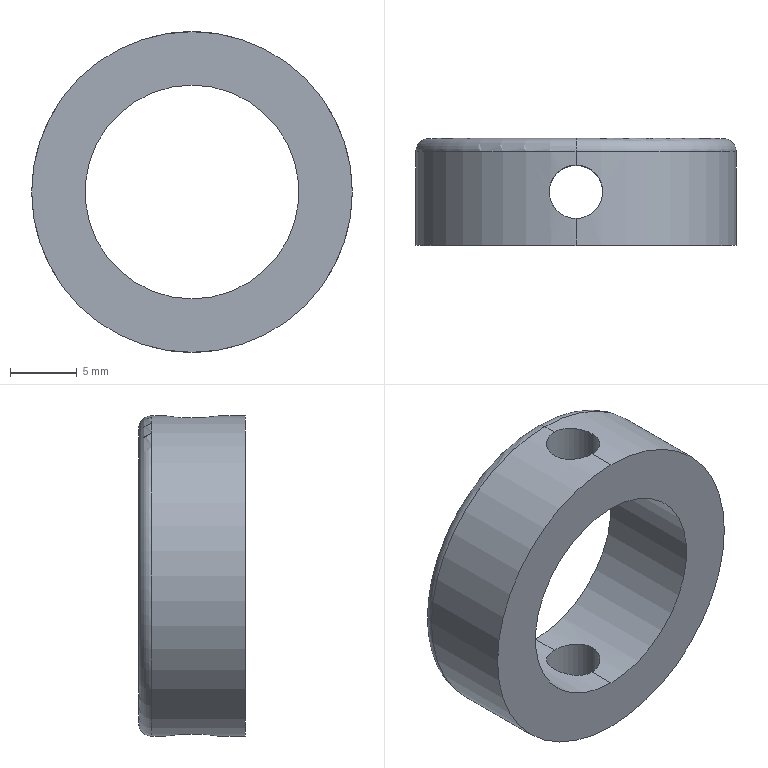Part | SolidWorks | features Extrusion 1, Fillet 1, ICE 1 | 1 solid | 12 faces | box 24 x 8 x 24 mm | volume 1894 mm3 | cylinder 8 | torus 2 | plane 2 | commonest cylinder face diameters 4 x4 16 x2 24 x2
STEP:
#1=CARTESIAN_POINT('',(0.,-1.,-12.));
#2=VERTEX_POINT('',#1);
#3=CARTESIAN_POINT('',(0.,-1.,12.));
#4=VERTEX_POINT('',#3);
#5=CARTESIAN_POINT('',(0.,-1.,0.));
#6=DIRECTION('',(0.,-1.,0.));
#7=DIRECTION('',(0.,0.,1.));
#8=AXIS2_PLACEMENT_3D('',#5,#6,#7);
#9=CIRCLE('',#8,12.);
#10=EDGE_CURVE('',#2,#4,#9,.T.);
#11=ORIENTED_EDGE('',*,*,#10,.F.);
#12=CARTESIAN_POINT('',(0.,0.,-11.));
#13=VERTEX_POINT('',#12);
#14=CARTESIAN_POINT('',(0.,-1.,-11.));
#15=DIRECTION('',(1.,0.,0.));
#16=DIRECTION('',(0.,0.,-1.));
#17=AXIS2_PLACEMENT_3D('',#14,#15,#16);
#18=CIRCLE('',#17,1.);
#19=EDGE_CURVE('',#2,#13,#18,.T.);
#20=ORIENTED_EDGE('',*,*,#19,.T.);
#21=CARTESIAN_POINT('',(0.,0.,11.));
#22=VERTEX_POINT('',#21);
#23=CARTESIAN_POINT('',(0.,0.,0.));
#24=DIRECTION('',(0.,1.,0.));
#25=DIRECTION('',(0.,0.,1.));
#26=AXIS2_PLACEMENT_3D('',#23,#24,#25);
#27=CIRCLE('',#26,11.);
#28=EDGE_CURVE('',#22,#13,#27,.T.);
#29=ORIENTED_EDGE('',*,*,#28,.F.);
#30=CARTESIAN_POINT('',(0.,-1.,11.));
#31=DIRECTION('',(-1.,0.,0.));
#32=DIRECTION('',(0.,0.,1.));
#33=AXIS2_PLACEMENT_3D('',#30,#31,#32);
#34=CIRCLE('',#33,1.);
#35=EDGE_CURVE('',#4,#22,#34,.T.);
#36=ORIENTED_EDGE('',*,*,#35,.F.);
#37=EDGE_LOOP('',(#11,#20,#29,#36));
#38=FACE_OUTER_BOUND('',#37,.T.);
#39=CARTESIAN_POINT('',(0.,-1.,0.));
#40=DIRECTION('',(0.,1.,0.));
#41=DIRECTION('',(0.,0.,1.));
#42=AXIS2_PLACEMENT_3D('',#39,#40,#41);
#43=TOROIDAL_SURFACE('',#42,11.,1.);
#44=ADVANCED_FACE('',(#38),#43,.T.);
#45=CARTESIAN_POINT('',(-2.,-4.,7.746));
#46=VERTEX_POINT('',#45);
#47=CARTESIAN_POINT('',(0.,-6.,8.));
#48=VERTEX_POINT('',#47);
#49=CARTESIAN_POINT('',(-2.,-4.,7.746));
#50=CARTESIAN_POINT('',(-2.,-4.132,7.746));
#51=CARTESIAN_POINT('',(-1.987,-4.262,7.749));
#52=CARTESIAN_POINT('',(-1.936,-4.519,7.762));
#53=CARTESIAN_POINT('',(-1.897,-4.646,7.772));
#54=CARTESIAN_POINT('',(-1.747,-5.008,7.808));
#55=CARTESIAN_POINT('',(-1.598,-5.23,7.841));
#56=CARTESIAN_POINT('',(-1.231,-5.597,7.907));
#57=CARTESIAN_POINT('',(-1.009,-5.746,7.94));
#58=CARTESIAN_POINT('',(-0.6485,-5.896,7.975));
#59=CARTESIAN_POINT('',(-0.5211,-5.935,7.984));
#60=CARTESIAN_POINT('',(-0.2634,-5.987,7.997));
#61=CARTESIAN_POINT('',(-0.1326,-6.,8.));
#62=CARTESIAN_POINT('',(0.,-6.,8.));
#63=B_SPLINE_CURVE_WITH_KNOTS('',3,(#49,#50,#51,#52,#53,#54,#55,#56,#57,#58,#59,#60,#61,#62),.UNSPECIFIED.,.F.,.F.,(4,2,2,2,2,2,4),(0.009417,0.009809,0.0102,0.01099,0.01177,0.01216,0.01255),.UNSPECIFIED.);
#64=EDGE_CURVE('',#46,#48,#63,.T.);
#65=ORIENTED_EDGE('',*,*,#64,.F.);
#66=CARTESIAN_POINT('',(-2.,-4.,11.832));
#67=VERTEX_POINT('',#66);
#68=CARTESIAN_POINT('',(-2.,-4.,-12.));
#69=DIRECTION('',(0.,0.,1.));
#70=VECTOR('',#69,1000.);
#71=LINE('',#68,#70);
#72=EDGE_CURVE('',#46,#67,#71,.T.);
#73=ORIENTED_EDGE('',*,*,#72,.T.);
#74=CARTESIAN_POINT('',(0.,-6.,12.));
#75=VERTEX_POINT('',#74);
#76=CARTESIAN_POINT('',(-2.,-4.,11.832));
#77=CARTESIAN_POINT('',(-2.,-4.132,11.832));
#78=CARTESIAN_POINT('',(-1.987,-4.262,11.834));
#79=CARTESIAN_POINT('',(-1.936,-4.518,11.843));
#80=CARTESIAN_POINT('',(-1.898,-4.645,11.849));
#81=CARTESIAN_POINT('',(-1.797,-4.887,11.865));
#82=CARTESIAN_POINT('',(-1.736,-5.002,11.874));
#83=CARTESIAN_POINT('',(-1.591,-5.219,11.894));
#84=CARTESIAN_POINT('',(-1.507,-5.322,11.905));
#85=CARTESIAN_POINT('',(-1.231,-5.598,11.938));
#86=CARTESIAN_POINT('',(-1.008,-5.747,11.96));
#87=CARTESIAN_POINT('',(-0.5275,-5.947,11.991));
#88=CARTESIAN_POINT('',(-0.2646,-6.,12.));
#89=CARTESIAN_POINT('',(0.,-6.,12.));
#90=B_SPLINE_CURVE_WITH_KNOTS('',3,(#76,#77,#78,#79,#80,#81,#82,#83,#84,#85,#86,#87,#88,#89),.UNSPECIFIED.,.F.,.F.,(4,2,2,2,2,2,4),(0.009396,0.009787,0.01018,0.01057,0.01096,0.01174,0.01253),.UNSPECIFIED.);
#91=EDGE_CURVE('',#67,#75,#90,.T.);
#92=ORIENTED_EDGE('',*,*,#91,.T.);
#93=CARTESIAN_POINT('',(2.,-4.,11.832));
#94=VERTEX_POINT('',#93);
#95=CARTESIAN_POINT('',(0.,-6.,12.));
#96=CARTESIAN_POINT('',(0.1324,-6.,12.));
#97=CARTESIAN_POINT('',(0.2626,-5.987,11.998));
#98=CARTESIAN_POINT('',(0.5186,-5.936,11.989));
#99=CARTESIAN_POINT('',(0.6458,-5.897,11.983));
#100=CARTESIAN_POINT('',(0.888,-5.797,11.968));
#101=CARTESIAN_POINT('',(1.003,-5.735,11.959));
#102=CARTESIAN_POINT('',(1.22,-5.59,11.938));
#103=CARTESIAN_POINT('',(1.323,-5.506,11.927));
#104=CARTESIAN_POINT('',(1.599,-5.229,11.894));
#105=CARTESIAN_POINT('',(1.748,-5.006,11.872));
#106=CARTESIAN_POINT('',(1.947,-4.525,11.841));
#107=CARTESIAN_POINT('',(2.,-4.261,11.832));
#108=CARTESIAN_POINT('',(2.,-4.,11.832));
#109=B_SPLINE_CURVE_WITH_KNOTS('',3,(#95,#96,#97,#98,#99,#100,#101,#102,#103,#104,#105,#106,#107,#108),.UNSPECIFIED.,.F.,.F.,(4,2,2,2,2,2,4),(0.,0.0003916,0.0007832,0.001175,0.001566,0.00235,0.003133),.UNSPECIFIED.);
#110=EDGE_CURVE('',#75,#94,#109,.T.);
#111=ORIENTED_EDGE('',*,*,#110,.T.);
#112=CARTESIAN_POINT('',(2.,-4.,7.746));
#113=VERTEX_POINT('',#112);
#114=CARTESIAN_POINT('',(2.,-4.,-12.));
#115=DIRECTION('',(0.,0.,1.));
#116=VECTOR('',#115,1000.);
#117=LINE('',#114,#116);
#118=EDGE_CURVE('',#113,#94,#117,.T.);
#119=ORIENTED_EDGE('',*,*,#118,.F.);
#120=CARTESIAN_POINT('',(0.,-6.,8.));
#121=CARTESIAN_POINT('',(0.1327,-6.,8.));
#122=CARTESIAN_POINT('',(0.2632,-5.987,7.997));
#123=CARTESIAN_POINT('',(0.5196,-5.936,7.984));
#124=CARTESIAN_POINT('',(0.647,-5.897,7.975));
#125=CARTESIAN_POINT('',(0.889,-5.796,7.951));
#126=CARTESIAN_POINT('',(1.004,-5.735,7.938));
#127=CARTESIAN_POINT('',(1.221,-5.59,7.907));
#128=CARTESIAN_POINT('',(1.323,-5.505,7.89));
#129=CARTESIAN_POINT('',(1.599,-5.23,7.841));
#130=CARTESIAN_POINT('',(1.747,-5.007,7.808));
#131=CARTESIAN_POINT('',(1.897,-4.646,7.772));
#132=CARTESIAN_POINT('',(1.936,-4.52,7.762));
#133=CARTESIAN_POINT('',(1.987,-4.261,7.749));
#134=CARTESIAN_POINT('',(2.,-4.131,7.746));
#135=CARTESIAN_POINT('',(2.,-4.,7.746));
#136=B_SPLINE_CURVE_WITH_KNOTS('',3,(#120,#121,#122,#123,#124,#125,#126,#127,#128,#129,#130,#131,#132,#133,#134,#135),.UNSPECIFIED.,.F.,.F.,(4,2,2,2,2,2,2,4),(0.,0.0003925,0.0007849,0.001177,0.00157,0.002355,0.002747,0.00314),.UNSPECIFIED.);
#137=EDGE_CURVE('',#48,#113,#136,.T.);
#138=ORIENTED_EDGE('',*,*,#137,.F.);
#139=EDGE_LOOP('',(#65,#73,#92,#111,#119,#138));
#140=FACE_OUTER_BOUND('',#139,.T.);
#141=CARTESIAN_POINT('',(0.,-4.,-12.));
#142=DIRECTION('',(0.,0.,1.));
#143=DIRECTION('',(1.,0.,0.));
#144=AXIS2_PLACEMENT_3D('',#141,#142,#143);
#145=CYLINDRICAL_SURFACE('',#144,2.);
#146=ADVANCED_FACE('',(#140),#145,.F.);
#147=CARTESIAN_POINT('',(0.,-6.,-12.));
#148=VERTEX_POINT('',#147);
#149=CARTESIAN_POINT('',(-2.,-4.,-11.832));
#150=VERTEX_POINT('',#149);
#151=CARTESIAN_POINT('',(0.,-6.,-12.));
#152=CARTESIAN_POINT('',(-0.2613,-6.,-12.));
#153=CARTESIAN_POINT('',(-0.525,-5.947,-11.991));
#154=CARTESIAN_POINT('',(-0.8862,-5.798,-11.968));
#155=CARTESIAN_POINT('',(-1.003,-5.735,-11.959));
#156=CARTESIAN_POINT('',(-1.221,-5.589,-11.938));
#157=CARTESIAN_POINT('',(-1.322,-5.507,-11.927));
#158=CARTESIAN_POINT('',(-1.506,-5.322,-11.905));
#159=CARTESIAN_POINT('',(-1.59,-5.22,-11.894));
#160=CARTESIAN_POINT('',(-1.735,-5.003,-11.874));
#161=CARTESIAN_POINT('',(-1.797,-4.888,-11.865));
#162=CARTESIAN_POINT('',(-1.898,-4.646,-11.849));
#163=CARTESIAN_POINT('',(-1.936,-4.519,-11.843));
#164=CARTESIAN_POINT('',(-1.987,-4.263,-11.834));
#165=CARTESIAN_POINT('',(-2.,-4.132,-11.832));
#166=CARTESIAN_POINT('',(-2.,-4.,-11.832));
#167=B_SPLINE_CURVE_WITH_KNOTS('',3,(#151,#152,#153,#154,#155,#156,#157,#158,#159,#160,#161,#162,#163,#164,#165,#166),.UNSPECIFIED.,.F.,.F.,(4,2,2,2,2,2,2,4),(0.006264,0.007047,0.007438,0.00783,0.008222,0.008613,0.009005,0.009396),.UNSPECIFIED.);
#168=EDGE_CURVE('',#148,#150,#167,.T.);
#169=ORIENTED_EDGE('',*,*,#168,.T.);
#170=CARTESIAN_POINT('',(-2.,-4.,-7.746));
#171=VERTEX_POINT('',#170);
#172=CARTESIAN_POINT('',(-2.,-4.,-12.));
#173=DIRECTION('',(0.,0.,1.));
#174=VECTOR('',#173,1000.);
#175=LINE('',#172,#174);
#176=EDGE_CURVE('',#150,#171,#175,.T.);
#177=ORIENTED_EDGE('',*,*,#176,.T.);
#178=CARTESIAN_POINT('',(0.,-6.,-8.));
#179=VERTEX_POINT('',#178);
#180=CARTESIAN_POINT('',(0.,-6.,-8.));
#181=CARTESIAN_POINT('',(-0.131,-6.,-8.));
#182=CARTESIAN_POINT('',(-0.2641,-5.987,-7.997));
#183=CARTESIAN_POINT('',(-0.521,-5.935,-7.984));
#184=CARTESIAN_POINT('',(-0.6459,-5.897,-7.975));
#185=CARTESIAN_POINT('',(-1.01,-5.746,-7.94));
#186=CARTESIAN_POINT('',(-1.23,-5.599,-7.907));
#187=CARTESIAN_POINT('',(-1.508,-5.321,-7.857));
#188=CARTESIAN_POINT('',(-1.59,-5.22,-7.841));
#189=CARTESIAN_POINT('',(-1.734,-5.004,-7.81));
#190=CARTESIAN_POINT('',(-1.797,-4.887,-7.796));
#191=CARTESIAN_POINT('',(-1.897,-4.646,-7.772));
#192=CARTESIAN_POINT('',(-1.935,-4.521,-7.762));
#193=CARTESIAN_POINT('',(-1.987,-4.264,-7.749));
#194=CARTESIAN_POINT('',(-2.,-4.131,-7.746));
#195=CARTESIAN_POINT('',(-2.,-4.,-7.746));
#196=B_SPLINE_CURVE_WITH_KNOTS('',3,(#180,#181,#182,#183,#184,#185,#186,#187,#188,#189,#190,#191,#192,#193,#194,#195),.UNSPECIFIED.,.F.,.F.,(4,2,2,2,2,2,2,4),(0.00314,0.003532,0.003924,0.004709,0.005101,0.005493,0.005886,0.006278),.UNSPECIFIED.);
#197=EDGE_CURVE('',#179,#171,#196,.T.);
#198=ORIENTED_EDGE('',*,*,#197,.F.);
#199=CARTESIAN_POINT('',(2.,-4.,-7.746));
#200=VERTEX_POINT('',#199);
#201=CARTESIAN_POINT('',(2.,-4.,-7.746));
#202=CARTESIAN_POINT('',(2.,-4.133,-7.746));
#203=CARTESIAN_POINT('',(1.987,-4.263,-7.749));
#204=CARTESIAN_POINT('',(1.936,-4.52,-7.762));
#205=CARTESIAN_POINT('',(1.897,-4.647,-7.772));
#206=CARTESIAN_POINT('',(1.796,-4.889,-7.796));
#207=CARTESIAN_POINT('',(1.735,-5.004,-7.81));
#208=CARTESIAN_POINT('',(1.59,-5.221,-7.841));
#209=CARTESIAN_POINT('',(1.506,-5.323,-7.858));
#210=CARTESIAN_POINT('',(1.23,-5.598,-7.907));
#211=CARTESIAN_POINT('',(1.007,-5.747,-7.94));
#212=CARTESIAN_POINT('',(0.6465,-5.897,-7.975));
#213=CARTESIAN_POINT('',(0.5198,-5.936,-7.984));
#214=CARTESIAN_POINT('',(0.2613,-5.987,-7.997));
#215=CARTESIAN_POINT('',(0.1311,-6.,-8.));
#216=CARTESIAN_POINT('',(0.,-6.,-8.));
#217=B_SPLINE_CURVE_WITH_KNOTS('',3,(#201,#202,#203,#204,#205,#206,#207,#208,#209,#210,#211,#212,#213,#214,#215,#216),.UNSPECIFIED.,.F.,.F.,(4,2,2,2,2,2,2,4),(0.,0.0003925,0.0007849,0.001177,0.00157,0.002355,0.002747,0.00314),.UNSPECIFIED.);
#218=EDGE_CURVE('',#200,#179,#217,.T.);
#219=ORIENTED_EDGE('',*,*,#218,.F.);
#220=CARTESIAN_POINT('',(2.,-4.,-11.832));
#221=VERTEX_POINT('',#220);
#222=CARTESIAN_POINT('',(2.,-4.,-12.));
#223=DIRECTION('',(0.,0.,1.));
#224=VECTOR('',#223,1000.);
#225=LINE('',#222,#224);
#226=EDGE_CURVE('',#221,#200,#225,.T.);
#227=ORIENTED_EDGE('',*,*,#226,.F.);
#228=CARTESIAN_POINT('',(2.,-4.,-11.832));
#229=CARTESIAN_POINT('',(2.,-4.131,-11.832));
#230=CARTESIAN_POINT('',(1.987,-4.263,-11.834));
#231=CARTESIAN_POINT('',(1.936,-4.52,-11.843));
#232=CARTESIAN_POINT('',(1.898,-4.645,-11.849));
#233=CARTESIAN_POINT('',(1.797,-4.887,-11.865));
#234=CARTESIAN_POINT('',(1.735,-5.004,-11.874));
#235=CARTESIAN_POINT('',(1.59,-5.22,-11.894));
#236=CARTESIAN_POINT('',(1.507,-5.321,-11.905));
#237=CARTESIAN_POINT('',(1.321,-5.508,-11.927));
#238=CARTESIAN_POINT('',(1.22,-5.59,-11.938));
#239=CARTESIAN_POINT('',(1.004,-5.735,-11.958));
#240=CARTESIAN_POINT('',(0.8866,-5.798,-11.968));
#241=CARTESIAN_POINT('',(0.6447,-5.898,-11.983));
#242=CARTESIAN_POINT('',(0.5201,-5.936,-11.989));
#243=CARTESIAN_POINT('',(0.2633,-5.987,-11.998));
#244=CARTESIAN_POINT('',(0.1306,-6.,-12.));
#245=CARTESIAN_POINT('',(0.,-6.,-12.));
#246=B_SPLINE_CURVE_WITH_KNOTS('',3,(#228,#229,#230,#231,#232,#233,#234,#235,#236,#237,#238,#239,#240,#241,#242,#243,#244,#245),.UNSPECIFIED.,.F.,.F.,(4,2,2,2,2,2,2,2,4),(0.003133,0.003524,0.003915,0.004307,0.004698,0.00509,0.005481,0.005872,0.006264),.UNSPECIFIED.);
#247=EDGE_CURVE('',#221,#148,#246,.T.);
#248=ORIENTED_EDGE('',*,*,#247,.T.);
#249=EDGE_LOOP('',(#169,#177,#198,#219,#227,#248));
#250=FACE_OUTER_BOUND('',#249,.T.);
#251=CARTESIAN_POINT('',(0.,-4.,-12.));
#252=DIRECTION('',(0.,0.,1.));
#253=DIRECTION('',(1.,0.,0.));
#254=AXIS2_PLACEMENT_3D('',#251,#252,#253);
#255=CYLINDRICAL_SURFACE('',#254,2.);
#256=ADVANCED_FACE('',(#250),#255,.F.);
#257=CARTESIAN_POINT('',(0.,-8.,-8.));
#258=VERTEX_POINT('',#257);
#259=CARTESIAN_POINT('',(0.,-8.,8.));
#260=VERTEX_POINT('',#259);
#261=CARTESIAN_POINT('',(0.,-8.,0.));
#262=DIRECTION('',(0.,1.,0.));
#263=DIRECTION('',(0.,0.,1.));
#264=AXIS2_PLACEMENT_3D('',#261,#262,#263);
#265=CIRCLE('',#264,8.);
#266=EDGE_CURVE('',#258,#260,#265,.T.);
#267=ORIENTED_EDGE('',*,*,#266,.F.);
#268=CARTESIAN_POINT('',(0.,-8.,-8.));
#269=DIRECTION('',(0.,1.,0.));
#270=VECTOR('',#269,1000.);
#271=LINE('',#268,#270);
#272=EDGE_CURVE('',#258,#179,#271,.T.);
#273=ORIENTED_EDGE('',*,*,#272,.T.);
#274=ORIENTED_EDGE('',*,*,#197,.T.);
#275=CARTESIAN_POINT('',(0.,-2.,-8.));
#276=VERTEX_POINT('',#275);
#277=CARTESIAN_POINT('',(-2.,-4.,-7.746));
#278=CARTESIAN_POINT('',(-2.,-3.738,-7.746));
#279=CARTESIAN_POINT('',(-1.947,-3.474,-7.76));
#280=CARTESIAN_POINT('',(-1.797,-3.113,-7.796));
#281=CARTESIAN_POINT('',(-1.735,-2.996,-7.81));
#282=CARTESIAN_POINT('',(-1.589,-2.779,-7.841));
#283=CARTESIAN_POINT('',(-1.507,-2.679,-7.857));
#284=CARTESIAN_POINT('',(-1.322,-2.494,-7.89));
#285=CARTESIAN_POINT('',(-1.22,-2.41,-7.907));
#286=CARTESIAN_POINT('',(-1.004,-2.265,-7.937));
#287=CARTESIAN_POINT('',(-0.8894,-2.204,-7.951));
#288=CARTESIAN_POINT('',(-0.5243,-2.052,-7.987));
#289=CARTESIAN_POINT('',(-0.2639,-2.,-8.));
#290=CARTESIAN_POINT('',(0.,-2.,-8.));
#291=B_SPLINE_CURVE_WITH_KNOTS('',3,(#277,#278,#279,#280,#281,#282,#283,#284,#285,#286,#287,#288,#289,#290),.UNSPECIFIED.,.F.,.F.,(4,2,2,2,2,2,4),(0.006278,0.007063,0.007455,0.007847,0.00824,0.008632,0.009417),.UNSPECIFIED.);
#292=EDGE_CURVE('',#171,#276,#291,.T.);
#293=ORIENTED_EDGE('',*,*,#292,.T.);
#294=CARTESIAN_POINT('',(0.,0.,-8.));
#295=VERTEX_POINT('',#294);
#296=CARTESIAN_POINT('',(0.,-8.,-8.));
#297=DIRECTION('',(0.,1.,0.));
#298=VECTOR('',#297,1000.);
#299=LINE('',#296,#298);
#300=EDGE_CURVE('',#276,#295,#299,.T.);
#301=ORIENTED_EDGE('',*,*,#300,.T.);
#302=CARTESIAN_POINT('',(0.,0.,8.));
#303=VERTEX_POINT('',#302);
#304=CARTESIAN_POINT('',(0.,0.,0.));
#305=DIRECTION('',(0.,1.,0.));
#306=DIRECTION('',(0.,0.,1.));
#307=AXIS2_PLACEMENT_3D('',#304,#305,#306);
#308=CIRCLE('',#307,8.);
#309=EDGE_CURVE('',#295,#303,#308,.T.);
#310=ORIENTED_EDGE('',*,*,#309,.T.);
#311=CARTESIAN_POINT('',(0.,-2.,8.));
#312=VERTEX_POINT('',#311);
#313=CARTESIAN_POINT('',(0.,-8.,8.));
#314=DIRECTION('',(0.,1.,0.));
#315=VECTOR('',#314,1000.);
#316=LINE('',#313,#315);
#317=EDGE_CURVE('',#312,#303,#316,.T.);
#318=ORIENTED_EDGE('',*,*,#317,.F.);
#319=CARTESIAN_POINT('',(0.,-2.,8.));
#320=CARTESIAN_POINT('',(-0.2617,-2.,8.));
#321=CARTESIAN_POINT('',(-0.5258,-2.053,7.986));
#322=CARTESIAN_POINT('',(-0.8872,-2.203,7.952));
#323=CARTESIAN_POINT('',(-1.004,-2.265,7.937));
#324=CARTESIAN_POINT('',(-1.221,-2.411,7.907));
#325=CARTESIAN_POINT('',(-1.322,-2.493,7.891));
#326=CARTESIAN_POINT('',(-1.506,-2.678,7.858));
#327=CARTESIAN_POINT('',(-1.59,-2.78,7.841));
#328=CARTESIAN_POINT('',(-1.735,-2.996,7.81));
#329=CARTESIAN_POINT('',(-1.796,-3.111,7.796));
#330=CARTESIAN_POINT('',(-1.948,-3.476,7.76));
#331=CARTESIAN_POINT('',(-2.,-3.736,7.746));
#332=CARTESIAN_POINT('',(-2.,-4.,7.746));
#333=B_SPLINE_CURVE_WITH_KNOTS('',3,(#319,#320,#321,#322,#323,#324,#325,#326,#327,#328,#329,#330,#331,#332),.UNSPECIFIED.,.F.,.F.,(4,2,2,2,2,2,4),(0.006278,0.007063,0.007455,0.007847,0.00824,0.008632,0.009417),.UNSPECIFIED.);
#334=EDGE_CURVE('',#312,#46,#333,.T.);
#335=ORIENTED_EDGE('',*,*,#334,.T.);
#336=ORIENTED_EDGE('',*,*,#64,.T.);
#337=CARTESIAN_POINT('',(0.,-8.,8.));
#338=DIRECTION('',(0.,1.,0.));
#339=VECTOR('',#338,1000.);
#340=LINE('',#337,#339);
#341=EDGE_CURVE('',#260,#48,#340,.T.);
#342=ORIENTED_EDGE('',*,*,#341,.F.);
#343=EDGE_LOOP('',(#267,#273,#274,#293,#301,#310,#318,#335,#336,#342));
#344=FACE_OUTER_BOUND('',#343,.T.);
#345=CARTESIAN_POINT('',(0.,-8.,0.));
#346=DIRECTION('',(0.,1.,0.));
#347=DIRECTION('',(0.,0.,1.));
#348=AXIS2_PLACEMENT_3D('',#345,#346,#347);
#349=CYLINDRICAL_SURFACE('',#348,8.);
#350=ADVANCED_FACE('',(#344),#349,.F.);
#351=CARTESIAN_POINT('',(0.,-8.,12.));
#352=VERTEX_POINT('',#351);
#353=CARTESIAN_POINT('',(0.,-8.,-12.));
#354=VERTEX_POINT('',#353);
#355=CARTESIAN_POINT('',(0.,-8.,0.));
#356=DIRECTION('',(0.,1.,0.));
#357=DIRECTION('',(0.,0.,1.));
#358=AXIS2_PLACEMENT_3D('',#355,#356,#357);
#359=CIRCLE('',#358,12.);
#360=EDGE_CURVE('',#352,#354,#359,.T.);
#361=ORIENTED_EDGE('',*,*,#360,.T.);
#362=CARTESIAN_POINT('',(0.,-8.,-12.));
#363=DIRECTION('',(0.,1.,0.));
#364=VECTOR('',#363,1000.);
#365=LINE('',#362,#364);
#366=EDGE_CURVE('',#354,#148,#365,.T.);
#367=ORIENTED_EDGE('',*,*,#366,.T.);
#368=ORIENTED_EDGE('',*,*,#247,.F.);
#369=CARTESIAN_POINT('',(0.,-2.,-12.));
#370=VERTEX_POINT('',#369);
#371=CARTESIAN_POINT('',(0.,-2.,-12.));
#372=CARTESIAN_POINT('',(0.1324,-2.,-12.));
#373=CARTESIAN_POINT('',(0.2626,-2.013,-11.998));
#374=CARTESIAN_POINT('',(0.5186,-2.064,-11.989));
#375=CARTESIAN_POINT('',(0.6458,-2.103,-11.983));
#376=CARTESIAN_POINT('',(0.888,-2.203,-11.968));
#377=CARTESIAN_POINT('',(1.003,-2.265,-11.959));
#378=CARTESIAN_POINT('',(1.22,-2.41,-11.938));
#379=CARTESIAN_POINT('',(1.323,-2.494,-11.927));
#380=CARTESIAN_POINT('',(1.599,-2.771,-11.894));
#381=CARTESIAN_POINT('',(1.748,-2.994,-11.872));
#382=CARTESIAN_POINT('',(1.947,-3.475,-11.841));
#383=CARTESIAN_POINT('',(2.,-3.739,-11.832));
#384=CARTESIAN_POINT('',(2.,-4.,-11.832));
#385=B_SPLINE_CURVE_WITH_KNOTS('',3,(#371,#372,#373,#374,#375,#376,#377,#378,#379,#380,#381,#382,#383,#384),.UNSPECIFIED.,.F.,.F.,(4,2,2,2,2,2,4),(0.,0.0003916,0.0007832,0.001175,0.001566,0.00235,0.003133),.UNSPECIFIED.);
#386=EDGE_CURVE('',#370,#221,#385,.T.);
#387=ORIENTED_EDGE('',*,*,#386,.F.);
#388=CARTESIAN_POINT('',(0.,-8.,-12.));
#389=DIRECTION('',(0.,1.,0.));
#390=VECTOR('',#389,1000.);
#391=LINE('',#388,#390);
#392=EDGE_CURVE('',#370,#2,#391,.T.);
#393=ORIENTED_EDGE('',*,*,#392,.T.);
#394=ORIENTED_EDGE('',*,*,#10,.T.);
#395=CARTESIAN_POINT('',(0.,-2.,12.));
#396=VERTEX_POINT('',#395);
#397=CARTESIAN_POINT('',(0.,-8.,12.));
#398=DIRECTION('',(0.,1.,0.));
#399=VECTOR('',#398,1000.);
#400=LINE('',#397,#399);
#401=EDGE_CURVE('',#396,#4,#400,.T.);
#402=ORIENTED_EDGE('',*,*,#401,.F.);
#403=CARTESIAN_POINT('',(2.,-4.,11.832));
#404=CARTESIAN_POINT('',(2.,-3.869,11.832));
#405=CARTESIAN_POINT('',(1.987,-3.737,11.834));
#406=CARTESIAN_POINT('',(1.936,-3.48,11.843));
#407=CARTESIAN_POINT('',(1.898,-3.355,11.849));
#408=CARTESIAN_POINT('',(1.797,-3.113,11.865));
#409=CARTESIAN_POINT('',(1.735,-2.996,11.874));
#410=CARTESIAN_POINT('',(1.59,-2.78,11.894));
#411=CARTESIAN_POINT('',(1.507,-2.679,11.905));
#412=CARTESIAN_POINT('',(1.321,-2.492,11.927));
#413=CARTESIAN_POINT('',(1.22,-2.41,11.938));
#414=CARTESIAN_POINT('',(1.004,-2.265,11.958));
#415=CARTESIAN_POINT('',(0.8866,-2.202,11.968));
#416=CARTESIAN_POINT('',(0.6447,-2.102,11.983));
#417=CARTESIAN_POINT('',(0.5201,-2.064,11.989));
#418=CARTESIAN_POINT('',(0.2633,-2.013,11.998));
#419=CARTESIAN_POINT('',(0.1306,-2.,12.));
#420=CARTESIAN_POINT('',(0.,-2.,12.));
#421=B_SPLINE_CURVE_WITH_KNOTS('',3,(#403,#404,#405,#406,#407,#408,#409,#410,#411,#412,#413,#414,#415,#416,#417,#418,#419,#420),.UNSPECIFIED.,.F.,.F.,(4,2,2,2,2,2,2,2,4),(0.003133,0.003524,0.003915,0.004307,0.004698,0.00509,0.005481,0.005872,0.006264),.UNSPECIFIED.);
#422=EDGE_CURVE('',#94,#396,#421,.T.);
#423=ORIENTED_EDGE('',*,*,#422,.F.);
#424=ORIENTED_EDGE('',*,*,#110,.F.);
#425=CARTESIAN_POINT('',(0.,-8.,12.));
#426=DIRECTION('',(0.,1.,0.));
#427=VECTOR('',#426,1000.);
#428=LINE('',#425,#427);
#429=EDGE_CURVE('',#352,#75,#428,.T.);
#430=ORIENTED_EDGE('',*,*,#429,.F.);
#431=EDGE_LOOP('',(#361,#367,#368,#387,#393,#394,#402,#423,#424,#430));
#432=FACE_OUTER_BOUND('',#431,.T.);
#433=CARTESIAN_POINT('',(0.,-8.,0.));
#434=DIRECTION('',(0.,1.,0.));
#435=DIRECTION('',(0.,0.,1.));
#436=AXIS2_PLACEMENT_3D('',#433,#434,#435);
#437=CYLINDRICAL_SURFACE('',#436,12.);
#438=ADVANCED_FACE('',(#432),#437,.T.);
#439=ORIENTED_EDGE('',*,*,#366,.F.);
#440=CARTESIAN_POINT('',(0.,-8.,0.));
#441=DIRECTION('',(0.,1.,0.));
#442=DIRECTION('',(0.,0.,1.));
#443=AXIS2_PLACEMENT_3D('',#440,#441,#442);
#444=CIRCLE('',#443,12.);
#445=EDGE_CURVE('',#354,#352,#444,.T.);
#446=ORIENTED_EDGE('',*,*,#445,.T.);
#447=ORIENTED_EDGE('',*,*,#429,.T.);
#448=ORIENTED_EDGE('',*,*,#91,.F.);
#449=CARTESIAN_POINT('',(0.,-2.,12.));
#450=CARTESIAN_POINT('',(-0.2613,-2.,12.));
#451=CARTESIAN_POINT('',(-0.525,-2.053,11.991));
#452=CARTESIAN_POINT('',(-0.8862,-2.202,11.968));
#453=CARTESIAN_POINT('',(-1.003,-2.265,11.959));
#454=CARTESIAN_POINT('',(-1.221,-2.411,11.938));
#455=CARTESIAN_POINT('',(-1.322,-2.493,11.927));
#456=CARTESIAN_POINT('',(-1.506,-2.678,11.905));
#457=CARTESIAN_POINT('',(-1.59,-2.78,11.894));
#458=CARTESIAN_POINT('',(-1.735,-2.997,11.874));
#459=CARTESIAN_POINT('',(-1.797,-3.112,11.865));
#460=CARTESIAN_POINT('',(-1.898,-3.354,11.849));
#461=CARTESIAN_POINT('',(-1.936,-3.481,11.843));
#462=CARTESIAN_POINT('',(-1.987,-3.737,11.834));
#463=CARTESIAN_POINT('',(-2.,-3.868,11.832));
#464=CARTESIAN_POINT('',(-2.,-4.,11.832));
#465=B_SPLINE_CURVE_WITH_KNOTS('',3,(#449,#450,#451,#452,#453,#454,#455,#456,#457,#458,#459,#460,#461,#462,#463,#464),.UNSPECIFIED.,.F.,.F.,(4,2,2,2,2,2,2,4),(0.006264,0.007047,0.007438,0.00783,0.008222,0.008613,0.009005,0.009396),.UNSPECIFIED.);
#466=EDGE_CURVE('',#396,#67,#465,.T.);
#467=ORIENTED_EDGE('',*,*,#466,.F.);
#468=ORIENTED_EDGE('',*,*,#401,.T.);
#469=CARTESIAN_POINT('',(0.,-1.,0.));
#470=DIRECTION('',(0.,-1.,0.));
#471=DIRECTION('',(0.,0.,1.));
#472=AXIS2_PLACEMENT_3D('',#469,#470,#471);
#473=CIRCLE('',#472,12.);
#474=EDGE_CURVE('',#4,#2,#473,.T.);
#475=ORIENTED_EDGE('',*,*,#474,.T.);
#476=ORIENTED_EDGE('',*,*,#392,.F.);
#477=CARTESIAN_POINT('',(-2.,-4.,-11.832));
#478=CARTESIAN_POINT('',(-2.,-3.868,-11.832));
#479=CARTESIAN_POINT('',(-1.987,-3.738,-11.834));
#480=CARTESIAN_POINT('',(-1.936,-3.482,-11.843));
#481=CARTESIAN_POINT('',(-1.898,-3.355,-11.849));
#482=CARTESIAN_POINT('',(-1.797,-3.113,-11.865));
#483=CARTESIAN_POINT('',(-1.736,-2.998,-11.874));
#484=CARTESIAN_POINT('',(-1.591,-2.781,-11.894));
#485=CARTESIAN_POINT('',(-1.507,-2.678,-11.905));
#486=CARTESIAN_POINT('',(-1.231,-2.402,-11.938));
#487=CARTESIAN_POINT('',(-1.008,-2.253,-11.96));
#488=CARTESIAN_POINT('',(-0.5275,-2.053,-11.991));
#489=CARTESIAN_POINT('',(-0.2646,-2.,-12.));
#490=CARTESIAN_POINT('',(0.,-2.,-12.));
#491=B_SPLINE_CURVE_WITH_KNOTS('',3,(#477,#478,#479,#480,#481,#482,#483,#484,#485,#486,#487,#488,#489,#490),.UNSPECIFIED.,.F.,.F.,(4,2,2,2,2,2,4),(0.009396,0.009787,0.01018,0.01057,0.01096,0.01174,0.01253),.UNSPECIFIED.);
#492=EDGE_CURVE('',#150,#370,#491,.T.);
#493=ORIENTED_EDGE('',*,*,#492,.F.);
#494=ORIENTED_EDGE('',*,*,#168,.F.);
#495=EDGE_LOOP('',(#439,#446,#447,#448,#467,#468,#475,#476,#493,#494));
#496=FACE_OUTER_BOUND('',#495,.T.);
#497=CARTESIAN_POINT('',(0.,-8.,0.));
#498=DIRECTION('',(0.,1.,0.));
#499=DIRECTION('',(0.,0.,1.));
#500=AXIS2_PLACEMENT_3D('',#497,#498,#499);
#501=CYLINDRICAL_SURFACE('',#500,12.);
#502=ADVANCED_FACE('',(#496),#501,.T.);
#503=CARTESIAN_POINT('',(0.,-8.,0.));
#504=DIRECTION('',(0.,1.,0.));
#505=DIRECTION('',(0.,0.,1.));
#506=AXIS2_PLACEMENT_3D('',#503,#504,#505);
#507=CIRCLE('',#506,8.);
#508=EDGE_CURVE('',#260,#258,#507,.T.);
#509=ORIENTED_EDGE('',*,*,#508,.T.);
#510=ORIENTED_EDGE('',*,*,#266,.T.);
#511=EDGE_LOOP('',(#509,#510));
#512=FACE_BOUND('',#511,.T.);
#513=ORIENTED_EDGE('',*,*,#360,.F.);
#514=ORIENTED_EDGE('',*,*,#445,.F.);
#515=EDGE_LOOP('',(#513,#514));
#516=FACE_OUTER_BOUND('',#515,.T.);
#517=CARTESIAN_POINT('',(0.,-8.,0.));
#518=DIRECTION('',(0.,1.,0.));
#519=DIRECTION('',(0.,0.,1.));
#520=AXIS2_PLACEMENT_3D('',#517,#518,#519);
#521=PLANE('',#520);
#522=ADVANCED_FACE('',(#512,#516),#521,.F.);
#523=ORIENTED_EDGE('',*,*,#28,.T.);
#524=CARTESIAN_POINT('',(0.,0.,0.));
#525=DIRECTION('',(0.,1.,0.));
#526=DIRECTION('',(0.,0.,1.));
#527=AXIS2_PLACEMENT_3D('',#524,#525,#526);
#528=CIRCLE('',#527,11.);
#529=EDGE_CURVE('',#13,#22,#528,.T.);
#530=ORIENTED_EDGE('',*,*,#529,.T.);
#531=EDGE_LOOP('',(#523,#530));
#532=FACE_OUTER_BOUND('',#531,.T.);
#533=CARTESIAN_POINT('',(0.,0.,0.));
#534=DIRECTION('',(0.,1.,0.));
#535=DIRECTION('',(0.,0.,1.));
#536=AXIS2_PLACEMENT_3D('',#533,#534,#535);
#537=CIRCLE('',#536,8.);
#538=EDGE_CURVE('',#303,#295,#537,.T.);
#539=ORIENTED_EDGE('',*,*,#538,.F.);
#540=ORIENTED_EDGE('',*,*,#309,.F.);
#541=EDGE_LOOP('',(#539,#540));
#542=FACE_BOUND('',#541,.T.);
#543=CARTESIAN_POINT('',(0.,0.,0.));
#544=DIRECTION('',(0.,1.,0.));
#545=DIRECTION('',(0.,0.,1.));
#546=AXIS2_PLACEMENT_3D('',#543,#544,#545);
#547=PLANE('',#546);
#548=ADVANCED_FACE('',(#532,#542),#547,.T.);
#549=ORIENTED_EDGE('',*,*,#272,.F.);
#550=ORIENTED_EDGE('',*,*,#508,.F.);
#551=ORIENTED_EDGE('',*,*,#341,.T.);
#552=ORIENTED_EDGE('',*,*,#137,.T.);
#553=CARTESIAN_POINT('',(2.,-4.,7.746));
#554=CARTESIAN_POINT('',(2.,-3.869,7.746));
#555=CARTESIAN_POINT('',(1.987,-3.736,7.749));
#556=CARTESIAN_POINT('',(1.935,-3.479,7.762));
#557=CARTESIAN_POINT('',(1.897,-3.354,7.772));
#558=CARTESIAN_POINT('',(1.746,-2.99,7.808));
#559=CARTESIAN_POINT('',(1.599,-2.77,7.841));
#560=CARTESIAN_POINT('',(1.321,-2.493,7.891));
#561=CARTESIAN_POINT('',(1.221,-2.41,7.907));
#562=CARTESIAN_POINT('',(1.004,-2.266,7.937));
#563=CARTESIAN_POINT('',(0.8872,-2.203,7.952));
#564=CARTESIAN_POINT('',(0.6458,-2.103,7.975));
#565=CARTESIAN_POINT('',(0.5211,-2.065,7.984));
#566=CARTESIAN_POINT('',(0.2636,-2.013,7.997));
#567=CARTESIAN_POINT('',(0.1308,-2.,8.));
#568=CARTESIAN_POINT('',(0.,-2.,8.));
#569=B_SPLINE_CURVE_WITH_KNOTS('',3,(#553,#554,#555,#556,#557,#558,#559,#560,#561,#562,#563,#564,#565,#566,#567,#568),.UNSPECIFIED.,.F.,.F.,(4,2,2,2,2,2,2,4),(0.00314,0.003532,0.003924,0.004709,0.005101,0.005493,0.005886,0.006278),.UNSPECIFIED.);
#570=EDGE_CURVE('',#113,#312,#569,.T.);
#571=ORIENTED_EDGE('',*,*,#570,.T.);
#572=ORIENTED_EDGE('',*,*,#317,.T.);
#573=ORIENTED_EDGE('',*,*,#538,.T.);
#574=ORIENTED_EDGE('',*,*,#300,.F.);
#575=CARTESIAN_POINT('',(0.,-2.,-8.));
#576=CARTESIAN_POINT('',(0.1319,-2.,-8.));
#577=CARTESIAN_POINT('',(0.262,-2.013,-7.997));
#578=CARTESIAN_POINT('',(0.5188,-2.064,-7.984));
#579=CARTESIAN_POINT('',(0.6465,-2.103,-7.975));
#580=CARTESIAN_POINT('',(1.008,-2.253,-7.94));
#581=CARTESIAN_POINT('',(1.23,-2.402,-7.907));
#582=CARTESIAN_POINT('',(1.597,-2.769,-7.841));
#583=CARTESIAN_POINT('',(1.746,-2.991,-7.808));
#584=CARTESIAN_POINT('',(1.896,-3.352,-7.772));
#585=CARTESIAN_POINT('',(1.935,-3.479,-7.762));
#586=CARTESIAN_POINT('',(1.987,-3.737,-7.749));
#587=CARTESIAN_POINT('',(2.,-3.867,-7.746));
#588=CARTESIAN_POINT('',(2.,-4.,-7.746));
#589=B_SPLINE_CURVE_WITH_KNOTS('',3,(#575,#576,#577,#578,#579,#580,#581,#582,#583,#584,#585,#586,#587,#588),.UNSPECIFIED.,.F.,.F.,(4,2,2,2,2,2,4),(0.009417,0.009809,0.0102,0.01099,0.01177,0.01216,0.01255),.UNSPECIFIED.);
#590=EDGE_CURVE('',#276,#200,#589,.T.);
#591=ORIENTED_EDGE('',*,*,#590,.T.);
#592=ORIENTED_EDGE('',*,*,#218,.T.);
#593=EDGE_LOOP('',(#549,#550,#551,#552,#571,#572,#573,#574,#591,#592));
#594=FACE_OUTER_BOUND('',#593,.T.);
#595=CARTESIAN_POINT('',(0.,-8.,0.));
#596=DIRECTION('',(0.,1.,0.));
#597=DIRECTION('',(0.,0.,1.));
#598=AXIS2_PLACEMENT_3D('',#595,#596,#597);
#599=CYLINDRICAL_SURFACE('',#598,8.);
#600=ADVANCED_FACE('',(#594),#599,.F.);
#601=ORIENTED_EDGE('',*,*,#176,.F.);
#602=ORIENTED_EDGE('',*,*,#492,.T.);
#603=ORIENTED_EDGE('',*,*,#386,.T.);
#604=ORIENTED_EDGE('',*,*,#226,.T.);
#605=ORIENTED_EDGE('',*,*,#590,.F.);
#606=ORIENTED_EDGE('',*,*,#292,.F.);
#607=EDGE_LOOP('',(#601,#602,#603,#604,#605,#606));
#608=FACE_OUTER_BOUND('',#607,.T.);
#609=CARTESIAN_POINT('',(0.,-4.,-12.));
#610=DIRECTION('',(0.,0.,1.));
#611=DIRECTION('',(1.,0.,0.));
#612=AXIS2_PLACEMENT_3D('',#609,#610,#611);
#613=CYLINDRICAL_SURFACE('',#612,2.);
#614=ADVANCED_FACE('',(#608),#613,.F.);
#615=ORIENTED_EDGE('',*,*,#72,.F.);
#616=ORIENTED_EDGE('',*,*,#334,.F.);
#617=ORIENTED_EDGE('',*,*,#570,.F.);
#618=ORIENTED_EDGE('',*,*,#118,.T.);
#619=ORIENTED_EDGE('',*,*,#422,.T.);
#620=ORIENTED_EDGE('',*,*,#466,.T.);
#621=EDGE_LOOP('',(#615,#616,#617,#618,#619,#620));
#622=FACE_OUTER_BOUND('',#621,.T.);
#623=CARTESIAN_POINT('',(0.,-4.,-12.));
#624=DIRECTION('',(0.,0.,1.));
#625=DIRECTION('',(1.,0.,0.));
#626=AXIS2_PLACEMENT_3D('',#623,#624,#625);
#627=CYLINDRICAL_SURFACE('',#626,2.);
#628=ADVANCED_FACE('',(#622),#627,.F.);
#629=ORIENTED_EDGE('',*,*,#19,.F.);
#630=ORIENTED_EDGE('',*,*,#474,.F.);
#631=ORIENTED_EDGE('',*,*,#35,.T.);
#632=ORIENTED_EDGE('',*,*,#529,.F.);
#633=EDGE_LOOP('',(#629,#630,#631,#632));
#634=FACE_OUTER_BOUND('',#633,.T.);
#635=CARTESIAN_POINT('',(0.,-1.,0.));
#636=DIRECTION('',(0.,1.,0.));
#637=DIRECTION('',(0.,0.,1.));
#638=AXIS2_PLACEMENT_3D('',#635,#636,#637);
#639=TOROIDAL_SURFACE('',#638,11.,1.);
#640=ADVANCED_FACE('',(#634),#639,.T.);
#641=CLOSED_SHELL('',(#44,#146,#256,#350,#438,#502,#522,#548,#600,#614,#628,#640));
#642=MANIFOLD_SOLID_BREP('',#641);
#643=CARTESIAN_POINT('',(0.,0.,0.));
#644=DIRECTION('',(0.,0.,1.));
#645=DIRECTION('',(1.,0.,0.));
#646=AXIS2_PLACEMENT_3D('',#643,#644,#645);
#647=(LENGTH_UNIT()NAMED_UNIT(*)SI_UNIT(.MILLI.,.METRE.));
#648=UNCERTAINTY_MEASURE_WITH_UNIT(LENGTH_MEASURE(0.00001),#647,'','');
#649=(NAMED_UNIT(*)PLANE_ANGLE_UNIT()SI_UNIT($,.RADIAN.));
#650=(NAMED_UNIT(*)SI_UNIT($,.STERADIAN.)SOLID_ANGLE_UNIT());
#651=(GEOMETRIC_REPRESENTATION_CONTEXT(3)GLOBAL_UNCERTAINTY_ASSIGNED_CONTEXT((#648))GLOBAL_UNIT_ASSIGNED_CONTEXT((#647,#649,#650))REPRESENTATION_CONTEXT('',''));
#652=ADVANCED_BREP_SHAPE_REPRESENTATION('',(#642,#646),#651);